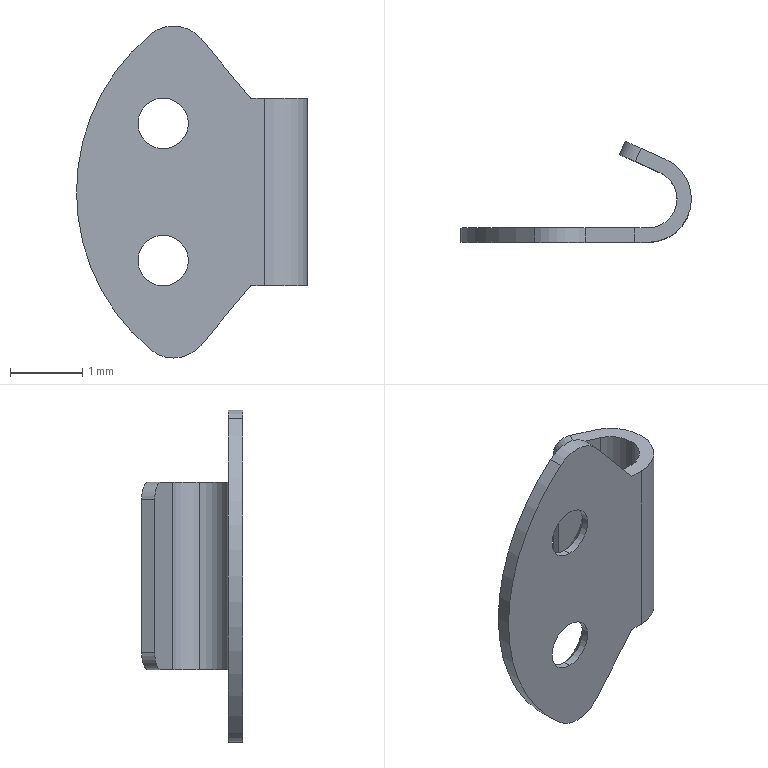Part | SolidWorks | features BaseBody 1, Scale 1 | 1 solid | 27 faces | box 3.2 x 1.4 x 4.6 mm | volume 2.668 mm3 | cylinder 14 | plane 9 | cone 4 | commonest cylinder face diameters 0.7 x4 1 x3 0.48 x2 0.8 x2 1.2 x2 5.686 x1
STEP:
#1=CARTESIAN_POINT('',(-19.88,-47.67,-12.1));
#2=VERTEX_POINT('',#1);
#3=CARTESIAN_POINT('',(-19.88,-47.67,-12.8));
#4=VERTEX_POINT('',#3);
#5=CARTESIAN_POINT('',(-19.88,-47.67,-12.45));
#6=DIRECTION('',(0.,-1.,0.));
#7=DIRECTION('',(0.,0.,1.));
#8=AXIS2_PLACEMENT_3D('',#5,#6,#7);
#9=CIRCLE('',#8,0.35);
#10=EDGE_CURVE('',#2,#4,#9,.T.);
#11=ORIENTED_EDGE('',*,*,#10,.T.);
#12=CARTESIAN_POINT('',(-19.88,-47.57,-12.9));
#13=VERTEX_POINT('',#12);
#14=CARTESIAN_POINT('',(-19.88,-47.67,-12.8));
#15=DIRECTION('',(0.,0.7071,-0.7071));
#16=VECTOR('',#15,1000.);
#17=LINE('',#14,#16);
#18=EDGE_CURVE('',#4,#13,#17,.T.);
#19=ORIENTED_EDGE('',*,*,#18,.T.);
#20=CARTESIAN_POINT('',(-19.88,-47.57,-12.));
#21=VERTEX_POINT('',#20);
#22=CARTESIAN_POINT('',(-19.88,-47.57,-12.45));
#23=DIRECTION('',(0.,1.,0.));
#24=DIRECTION('',(0.,0.,1.));
#25=AXIS2_PLACEMENT_3D('',#22,#23,#24);
#26=CIRCLE('',#25,0.45);
#27=EDGE_CURVE('',#13,#21,#26,.T.);
#28=ORIENTED_EDGE('',*,*,#27,.T.);
#29=CARTESIAN_POINT('',(-19.88,-47.67,-12.1));
#30=DIRECTION('',(0.,0.7071,0.7071));
#31=VECTOR('',#30,1000.);
#32=LINE('',#29,#31);
#33=EDGE_CURVE('',#2,#21,#32,.T.);
#34=ORIENTED_EDGE('',*,*,#33,.F.);
#35=EDGE_LOOP('',(#11,#19,#28,#34));
#36=FACE_OUTER_BOUND('',#35,.T.);
#37=CARTESIAN_POINT('',(-19.88,-47.67,-12.45));
#38=DIRECTION('',(0.,1.,0.));
#39=DIRECTION('',(0.,0.,1.));
#40=AXIS2_PLACEMENT_3D('',#37,#38,#39);
#41=CONICAL_SURFACE('',#40,0.35,0.7854);
#42=ADVANCED_FACE('',(#36),#41,.F.);
#43=ORIENTED_EDGE('',*,*,#10,.F.);
#44=CARTESIAN_POINT('',(-19.88,-47.77,-12.1));
#45=VERTEX_POINT('',#44);
#46=CARTESIAN_POINT('',(-19.88,-47.67,-12.1));
#47=DIRECTION('',(0.,-1.,0.));
#48=VECTOR('',#47,1000.);
#49=LINE('',#46,#48);
#50=EDGE_CURVE('',#2,#45,#49,.T.);
#51=ORIENTED_EDGE('',*,*,#50,.T.);
#52=CARTESIAN_POINT('',(-19.88,-47.77,-12.8));
#53=VERTEX_POINT('',#52);
#54=CARTESIAN_POINT('',(-19.88,-47.77,-12.45));
#55=DIRECTION('',(0.,-1.,0.));
#56=DIRECTION('',(0.,0.,-1.));
#57=AXIS2_PLACEMENT_3D('',#54,#55,#56);
#58=CIRCLE('',#57,0.35);
#59=EDGE_CURVE('',#45,#53,#58,.T.);
#60=ORIENTED_EDGE('',*,*,#59,.T.);
#61=CARTESIAN_POINT('',(-19.88,-47.67,-12.8));
#62=DIRECTION('',(0.,-1.,0.));
#63=VECTOR('',#62,1000.);
#64=LINE('',#61,#63);
#65=EDGE_CURVE('',#4,#53,#64,.T.);
#66=ORIENTED_EDGE('',*,*,#65,.F.);
#67=EDGE_LOOP('',(#43,#51,#60,#66));
#68=FACE_OUTER_BOUND('',#67,.T.);
#69=CARTESIAN_POINT('',(-19.88,-47.67,-12.45));
#70=DIRECTION('',(0.,-1.,0.));
#71=DIRECTION('',(0.,0.,-1.));
#72=AXIS2_PLACEMENT_3D('',#69,#70,#71);
#73=CYLINDRICAL_SURFACE('',#72,0.35);
#74=ADVANCED_FACE('',(#68),#73,.F.);
#75=CARTESIAN_POINT('',(-19.88,-47.67,-10.2));
#76=VERTEX_POINT('',#75);
#77=CARTESIAN_POINT('',(-19.88,-47.67,-10.9));
#78=VERTEX_POINT('',#77);
#79=CARTESIAN_POINT('',(-19.88,-47.67,-10.55));
#80=DIRECTION('',(0.,-1.,0.));
#81=DIRECTION('',(0.,0.,1.));
#82=AXIS2_PLACEMENT_3D('',#79,#80,#81);
#83=CIRCLE('',#82,0.35);
#84=EDGE_CURVE('',#76,#78,#83,.T.);
#85=ORIENTED_EDGE('',*,*,#84,.T.);
#86=CARTESIAN_POINT('',(-19.88,-47.57,-11.));
#87=VERTEX_POINT('',#86);
#88=CARTESIAN_POINT('',(-19.88,-47.67,-10.9));
#89=DIRECTION('',(0.,0.7071,-0.7071));
#90=VECTOR('',#89,1000.);
#91=LINE('',#88,#90);
#92=EDGE_CURVE('',#78,#87,#91,.T.);
#93=ORIENTED_EDGE('',*,*,#92,.T.);
#94=CARTESIAN_POINT('',(-19.88,-47.57,-10.1));
#95=VERTEX_POINT('',#94);
#96=CARTESIAN_POINT('',(-19.88,-47.57,-10.55));
#97=DIRECTION('',(0.,-1.,0.));
#98=DIRECTION('',(0.,0.,1.));
#99=AXIS2_PLACEMENT_3D('',#96,#97,#98);
#100=CIRCLE('',#99,0.45);
#101=EDGE_CURVE('',#95,#87,#100,.T.);
#102=ORIENTED_EDGE('',*,*,#101,.F.);
#103=CARTESIAN_POINT('',(-19.88,-47.67,-10.2));
#104=DIRECTION('',(0.,0.7071,0.7071));
#105=VECTOR('',#104,1000.);
#106=LINE('',#103,#105);
#107=EDGE_CURVE('',#76,#95,#106,.T.);
#108=ORIENTED_EDGE('',*,*,#107,.F.);
#109=EDGE_LOOP('',(#85,#93,#102,#108));
#110=FACE_OUTER_BOUND('',#109,.T.);
#111=CARTESIAN_POINT('',(-19.88,-47.67,-10.55));
#112=DIRECTION('',(0.,1.,0.));
#113=DIRECTION('',(0.,0.,1.));
#114=AXIS2_PLACEMENT_3D('',#111,#112,#113);
#115=CONICAL_SURFACE('',#114,0.35,0.7854);
#116=ADVANCED_FACE('',(#110),#115,.F.);
#117=CARTESIAN_POINT('',(-18.317,-46.805,-12.8));
#118=VERTEX_POINT('',#117);
#119=CARTESIAN_POINT('',(-18.08,-47.17,-12.8));
#120=VERTEX_POINT('',#119);
#121=CARTESIAN_POINT('',(-18.48,-47.17,-12.8));
#122=DIRECTION('',(0.,0.,-1.));
#123=DIRECTION('',(1.,0.,0.));
#124=AXIS2_PLACEMENT_3D('',#121,#122,#123);
#125=CIRCLE('',#124,0.4);
#126=EDGE_CURVE('',#118,#120,#125,.T.);
#127=ORIENTED_EDGE('',*,*,#126,.T.);
#128=CARTESIAN_POINT('',(-18.08,-47.17,-10.2));
#129=VERTEX_POINT('',#128);
#130=CARTESIAN_POINT('',(-18.08,-47.17,-12.8));
#131=DIRECTION('',(0.,0.,1.));
#132=VECTOR('',#131,1000.);
#133=LINE('',#130,#132);
#134=EDGE_CURVE('',#120,#129,#133,.T.);
#135=ORIENTED_EDGE('',*,*,#134,.T.);
#136=CARTESIAN_POINT('',(-18.317,-46.805,-10.2));
#137=VERTEX_POINT('',#136);
#138=CARTESIAN_POINT('',(-18.48,-47.17,-10.2));
#139=DIRECTION('',(0.,0.,1.));
#140=DIRECTION('',(1.,0.,0.));
#141=AXIS2_PLACEMENT_3D('',#138,#139,#140);
#142=CIRCLE('',#141,0.4);
#143=EDGE_CURVE('',#129,#137,#142,.T.);
#144=ORIENTED_EDGE('',*,*,#143,.T.);
#145=CARTESIAN_POINT('',(-18.317,-46.805,-11.5));
#146=DIRECTION('',(0.,0.,-1.));
#147=VECTOR('',#146,1000.);
#148=LINE('',#145,#147);
#149=EDGE_CURVE('',#137,#118,#148,.T.);
#150=ORIENTED_EDGE('',*,*,#149,.T.);
#151=EDGE_LOOP('',(#127,#135,#144,#150));
#152=FACE_OUTER_BOUND('',#151,.T.);
#153=CARTESIAN_POINT('',(-18.48,-47.17,-12.8));
#154=DIRECTION('',(0.,0.,1.));
#155=DIRECTION('',(1.,0.,0.));
#156=AXIS2_PLACEMENT_3D('',#153,#154,#155);
#157=CYLINDRICAL_SURFACE('',#156,0.4);
#158=ADVANCED_FACE('',(#152),#157,.F.);
#159=CARTESIAN_POINT('',(-19.737,-47.57,-13.8));
#160=VERTEX_POINT('',#159);
#161=CARTESIAN_POINT('',(-20.057,-47.57,-13.684));
#162=VERTEX_POINT('',#161);
#163=CARTESIAN_POINT('',(-19.737,-47.57,-13.3));
#164=DIRECTION('',(0.,1.,0.));
#165=DIRECTION('',(0.,0.,-1.));
#166=AXIS2_PLACEMENT_3D('',#163,#164,#165);
#167=CIRCLE('',#166,0.5);
#168=EDGE_CURVE('',#160,#162,#167,.T.);
#169=ORIENTED_EDGE('',*,*,#168,.F.);
#170=CARTESIAN_POINT('',(-19.737,-47.77,-13.8));
#171=VERTEX_POINT('',#170);
#172=CARTESIAN_POINT('',(-19.737,-47.57,-13.8));
#173=DIRECTION('',(0.,-1.,0.));
#174=VECTOR('',#173,1000.);
#175=LINE('',#172,#174);
#176=EDGE_CURVE('',#160,#171,#175,.T.);
#177=ORIENTED_EDGE('',*,*,#176,.T.);
#178=CARTESIAN_POINT('',(-20.057,-47.77,-13.684));
#179=VERTEX_POINT('',#178);
#180=CARTESIAN_POINT('',(-19.737,-47.77,-13.3));
#181=DIRECTION('',(0.,-1.,0.));
#182=DIRECTION('',(0.,0.,-1.));
#183=AXIS2_PLACEMENT_3D('',#180,#181,#182);
#184=CIRCLE('',#183,0.5);
#185=EDGE_CURVE('',#179,#171,#184,.T.);
#186=ORIENTED_EDGE('',*,*,#185,.F.);
#187=CARTESIAN_POINT('',(-20.057,-47.67,-13.684));
#188=DIRECTION('',(0.,1.,0.));
#189=VECTOR('',#188,1000.);
#190=LINE('',#187,#189);
#191=EDGE_CURVE('',#179,#162,#190,.T.);
#192=ORIENTED_EDGE('',*,*,#191,.T.);
#193=EDGE_LOOP('',(#169,#177,#186,#192));
#194=FACE_OUTER_BOUND('',#193,.T.);
#195=CARTESIAN_POINT('',(-19.737,-47.57,-13.3));
#196=DIRECTION('',(0.,-1.,0.));
#197=DIRECTION('',(0.,0.,-1.));
#198=AXIS2_PLACEMENT_3D('',#195,#196,#197);
#199=CYLINDRICAL_SURFACE('',#198,0.5);
#200=ADVANCED_FACE('',(#194),#199,.T.);
#201=ORIENTED_EDGE('',*,*,#84,.F.);
#202=CARTESIAN_POINT('',(-19.88,-47.77,-10.2));
#203=VERTEX_POINT('',#202);
#204=CARTESIAN_POINT('',(-19.88,-47.67,-10.2));
#205=DIRECTION('',(0.,-1.,0.));
#206=VECTOR('',#205,1000.);
#207=LINE('',#204,#206);
#208=EDGE_CURVE('',#76,#203,#207,.T.);
#209=ORIENTED_EDGE('',*,*,#208,.T.);
#210=CARTESIAN_POINT('',(-19.88,-47.77,-10.9));
#211=VERTEX_POINT('',#210);
#212=CARTESIAN_POINT('',(-19.88,-47.77,-10.55));
#213=DIRECTION('',(0.,1.,0.));
#214=DIRECTION('',(0.,0.,-1.));
#215=AXIS2_PLACEMENT_3D('',#212,#213,#214);
#216=CIRCLE('',#215,0.35);
#217=EDGE_CURVE('',#211,#203,#216,.T.);
#218=ORIENTED_EDGE('',*,*,#217,.F.);
#219=CARTESIAN_POINT('',(-19.88,-47.67,-10.9));
#220=DIRECTION('',(0.,-1.,0.));
#221=VECTOR('',#220,1000.);
#222=LINE('',#219,#221);
#223=EDGE_CURVE('',#78,#211,#222,.T.);
#224=ORIENTED_EDGE('',*,*,#223,.F.);
#225=EDGE_LOOP('',(#201,#209,#218,#224));
#226=FACE_OUTER_BOUND('',#225,.T.);
#227=CARTESIAN_POINT('',(-19.88,-47.67,-10.55));
#228=DIRECTION('',(0.,-1.,0.));
#229=DIRECTION('',(0.,0.,-1.));
#230=AXIS2_PLACEMENT_3D('',#227,#228,#229);
#231=CYLINDRICAL_SURFACE('',#230,0.35);
#232=ADVANCED_FACE('',(#226),#231,.F.);
#233=CARTESIAN_POINT('',(-18.48,-47.77,-12.8));
#234=VERTEX_POINT('',#233);
#235=CARTESIAN_POINT('',(-17.88,-47.17,-12.8));
#236=VERTEX_POINT('',#235);
#237=CARTESIAN_POINT('',(-18.48,-47.17,-12.8));
#238=DIRECTION('',(0.,0.,1.));
#239=DIRECTION('',(1.,0.,0.));
#240=AXIS2_PLACEMENT_3D('',#237,#238,#239);
#241=CIRCLE('',#240,0.6);
#242=EDGE_CURVE('',#234,#236,#241,.T.);
#243=ORIENTED_EDGE('',*,*,#242,.T.);
#244=CARTESIAN_POINT('',(-17.88,-47.17,-10.2));
#245=VERTEX_POINT('',#244);
#246=CARTESIAN_POINT('',(-17.88,-47.17,-12.8));
#247=DIRECTION('',(0.,0.,1.));
#248=VECTOR('',#247,1000.);
#249=LINE('',#246,#248);
#250=EDGE_CURVE('',#236,#245,#249,.T.);
#251=ORIENTED_EDGE('',*,*,#250,.T.);
#252=CARTESIAN_POINT('',(-18.48,-47.77,-10.2));
#253=VERTEX_POINT('',#252);
#254=CARTESIAN_POINT('',(-18.48,-47.17,-10.2));
#255=DIRECTION('',(0.,0.,-1.));
#256=DIRECTION('',(1.,0.,0.));
#257=AXIS2_PLACEMENT_3D('',#254,#255,#256);
#258=CIRCLE('',#257,0.6);
#259=EDGE_CURVE('',#245,#253,#258,.T.);
#260=ORIENTED_EDGE('',*,*,#259,.T.);
#261=CARTESIAN_POINT('',(-18.48,-47.77,-11.5));
#262=DIRECTION('',(0.,0.,1.));
#263=VECTOR('',#262,1000.);
#264=LINE('',#261,#263);
#265=EDGE_CURVE('',#234,#253,#264,.T.);
#266=ORIENTED_EDGE('',*,*,#265,.F.);
#267=EDGE_LOOP('',(#243,#251,#260,#266));
#268=FACE_OUTER_BOUND('',#267,.T.);
#269=CARTESIAN_POINT('',(-18.48,-47.17,-12.8));
#270=DIRECTION('',(0.,0.,1.));
#271=DIRECTION('',(1.,0.,0.));
#272=AXIS2_PLACEMENT_3D('',#269,#270,#271);
#273=CYLINDRICAL_SURFACE('',#272,0.6);
#274=ADVANCED_FACE('',(#268),#273,.T.);
#275=ORIENTED_EDGE('',*,*,#18,.F.);
#276=CARTESIAN_POINT('',(-19.88,-47.67,-12.45));
#277=DIRECTION('',(0.,-1.,0.));
#278=DIRECTION('',(0.,0.,1.));
#279=AXIS2_PLACEMENT_3D('',#276,#277,#278);
#280=CIRCLE('',#279,0.35);
#281=EDGE_CURVE('',#4,#2,#280,.T.);
#282=ORIENTED_EDGE('',*,*,#281,.T.);
#283=ORIENTED_EDGE('',*,*,#33,.T.);
#284=CARTESIAN_POINT('',(-19.88,-47.57,-12.45));
#285=DIRECTION('',(0.,1.,0.));
#286=DIRECTION('',(0.,0.,1.));
#287=AXIS2_PLACEMENT_3D('',#284,#285,#286);
#288=CIRCLE('',#287,0.45);
#289=EDGE_CURVE('',#21,#13,#288,.T.);
#290=ORIENTED_EDGE('',*,*,#289,.T.);
#291=EDGE_LOOP('',(#275,#282,#283,#290));
#292=FACE_OUTER_BOUND('',#291,.T.);
#293=CARTESIAN_POINT('',(-19.88,-47.67,-12.45));
#294=DIRECTION('',(0.,1.,0.));
#295=DIRECTION('',(0.,0.,1.));
#296=AXIS2_PLACEMENT_3D('',#293,#294,#295);
#297=CONICAL_SURFACE('',#296,0.35,0.7854);
#298=ADVANCED_FACE('',(#292),#297,.F.);
#299=ORIENTED_EDGE('',*,*,#289,.F.);
#300=ORIENTED_EDGE('',*,*,#27,.F.);
#301=EDGE_LOOP('',(#299,#300));
#302=FACE_BOUND('',#301,.T.);
#303=ORIENTED_EDGE('',*,*,#101,.T.);
#304=CARTESIAN_POINT('',(-19.88,-47.57,-10.55));
#305=DIRECTION('',(0.,-1.,0.));
#306=DIRECTION('',(0.,0.,1.));
#307=AXIS2_PLACEMENT_3D('',#304,#305,#306);
#308=CIRCLE('',#307,0.45);
#309=EDGE_CURVE('',#87,#95,#308,.T.);
#310=ORIENTED_EDGE('',*,*,#309,.T.);
#311=EDGE_LOOP('',(#303,#310));
#312=FACE_BOUND('',#311,.T.);
#313=CARTESIAN_POINT('',(-18.665,-47.57,-10.2));
#314=VERTEX_POINT('',#313);
#315=CARTESIAN_POINT('',(-18.48,-47.57,-10.2));
#316=VERTEX_POINT('',#315);
#317=CARTESIAN_POINT('',(-18.27,-47.57,-10.2));
#318=DIRECTION('',(1.,0.,0.));
#319=VECTOR('',#318,1000.);
#320=LINE('',#317,#319);
#321=EDGE_CURVE('',#314,#316,#320,.T.);
#322=ORIENTED_EDGE('',*,*,#321,.T.);
#323=CARTESIAN_POINT('',(-18.48,-47.57,-12.8));
#324=VERTEX_POINT('',#323);
#325=CARTESIAN_POINT('',(-18.48,-47.57,-11.5));
#326=DIRECTION('',(0.,0.,-1.));
#327=VECTOR('',#326,1000.);
#328=LINE('',#325,#327);
#329=EDGE_CURVE('',#316,#324,#328,.T.);
#330=ORIENTED_EDGE('',*,*,#329,.T.);
#331=CARTESIAN_POINT('',(-18.665,-47.57,-12.8));
#332=VERTEX_POINT('',#331);
#333=CARTESIAN_POINT('',(-18.27,-47.57,-12.8));
#334=DIRECTION('',(-1.,0.,0.));
#335=VECTOR('',#334,1000.);
#336=LINE('',#333,#335);
#337=EDGE_CURVE('',#324,#332,#336,.T.);
#338=ORIENTED_EDGE('',*,*,#337,.T.);
#339=CARTESIAN_POINT('',(-19.354,-47.57,-13.621));
#340=VERTEX_POINT('',#339);
#341=CARTESIAN_POINT('',(-18.665,-47.57,-12.8));
#342=DIRECTION('',(-0.6428,0.,-0.766));
#343=VECTOR('',#342,1000.);
#344=LINE('',#341,#343);
#345=EDGE_CURVE('',#332,#340,#344,.T.);
#346=ORIENTED_EDGE('',*,*,#345,.T.);
#347=CARTESIAN_POINT('',(-19.737,-47.57,-13.3));
#348=DIRECTION('',(0.,1.,0.));
#349=DIRECTION('',(0.,0.,-1.));
#350=AXIS2_PLACEMENT_3D('',#347,#348,#349);
#351=CIRCLE('',#350,0.5);
#352=EDGE_CURVE('',#340,#160,#351,.T.);
#353=ORIENTED_EDGE('',*,*,#352,.T.);
#354=ORIENTED_EDGE('',*,*,#168,.T.);
#355=CARTESIAN_POINT('',(-20.057,-47.57,-9.316));
#356=VERTEX_POINT('',#355);
#357=CARTESIAN_POINT('',(-18.237,-47.57,-11.5));
#358=DIRECTION('',(0.,1.,0.));
#359=DIRECTION('',(0.,0.,-1.));
#360=AXIS2_PLACEMENT_3D('',#357,#358,#359);
#361=CIRCLE('',#360,2.843);
#362=EDGE_CURVE('',#162,#356,#361,.T.);
#363=ORIENTED_EDGE('',*,*,#362,.T.);
#364=CARTESIAN_POINT('',(-19.354,-47.57,-9.379));
#365=VERTEX_POINT('',#364);
#366=CARTESIAN_POINT('',(-19.737,-47.57,-9.7));
#367=DIRECTION('',(0.,1.,0.));
#368=DIRECTION('',(0.,0.,-1.));
#369=AXIS2_PLACEMENT_3D('',#366,#367,#368);
#370=CIRCLE('',#369,0.5);
#371=EDGE_CURVE('',#356,#365,#370,.T.);
#372=ORIENTED_EDGE('',*,*,#371,.T.);
#373=CARTESIAN_POINT('',(-19.354,-47.57,-9.379));
#374=DIRECTION('',(0.6428,0.,-0.766));
#375=VECTOR('',#374,1000.);
#376=LINE('',#373,#375);
#377=EDGE_CURVE('',#365,#314,#376,.T.);
#378=ORIENTED_EDGE('',*,*,#377,.T.);
#379=EDGE_LOOP('',(#322,#330,#338,#346,#353,#354,#363,#372,#378));
#380=FACE_OUTER_BOUND('',#379,.T.);
#381=CARTESIAN_POINT('',(-18.48,-47.57,-13.828));
#382=DIRECTION('',(0.,1.,0.));
#383=DIRECTION('',(-1.,0.,0.));
#384=AXIS2_PLACEMENT_3D('',#381,#382,#383);
#385=PLANE('',#384);
#386=ADVANCED_FACE('',(#302,#312,#380),#385,.T.);
#387=ORIENTED_EDGE('',*,*,#50,.F.);
#388=ORIENTED_EDGE('',*,*,#281,.F.);
#389=ORIENTED_EDGE('',*,*,#65,.T.);
#390=CARTESIAN_POINT('',(-19.88,-47.77,-12.45));
#391=DIRECTION('',(0.,-1.,0.));
#392=DIRECTION('',(0.,0.,-1.));
#393=AXIS2_PLACEMENT_3D('',#390,#391,#392);
#394=CIRCLE('',#393,0.35);
#395=EDGE_CURVE('',#53,#45,#394,.T.);
#396=ORIENTED_EDGE('',*,*,#395,.T.);
#397=EDGE_LOOP('',(#387,#388,#389,#396));
#398=FACE_OUTER_BOUND('',#397,.T.);
#399=CARTESIAN_POINT('',(-19.88,-47.67,-12.45));
#400=DIRECTION('',(0.,-1.,0.));
#401=DIRECTION('',(0.,0.,-1.));
#402=AXIS2_PLACEMENT_3D('',#399,#400,#401);
#403=CYLINDRICAL_SURFACE('',#402,0.35);
#404=ADVANCED_FACE('',(#398),#403,.F.);
#405=ORIENTED_EDGE('',*,*,#92,.F.);
#406=CARTESIAN_POINT('',(-19.88,-47.67,-10.55));
#407=DIRECTION('',(0.,-1.,0.));
#408=DIRECTION('',(0.,0.,1.));
#409=AXIS2_PLACEMENT_3D('',#406,#407,#408);
#410=CIRCLE('',#409,0.35);
#411=EDGE_CURVE('',#78,#76,#410,.T.);
#412=ORIENTED_EDGE('',*,*,#411,.T.);
#413=ORIENTED_EDGE('',*,*,#107,.T.);
#414=ORIENTED_EDGE('',*,*,#309,.F.);
#415=EDGE_LOOP('',(#405,#412,#413,#414));
#416=FACE_OUTER_BOUND('',#415,.T.);
#417=CARTESIAN_POINT('',(-19.88,-47.67,-10.55));
#418=DIRECTION('',(0.,1.,0.));
#419=DIRECTION('',(0.,0.,1.));
#420=AXIS2_PLACEMENT_3D('',#417,#418,#419);
#421=CONICAL_SURFACE('',#420,0.35,0.7854);
#422=ADVANCED_FACE('',(#416),#421,.F.);
#423=ORIENTED_EDGE('',*,*,#134,.F.);
#424=CARTESIAN_POINT('',(-18.48,-47.17,-12.8));
#425=DIRECTION('',(0.,0.,-1.));
#426=DIRECTION('',(1.,0.,0.));
#427=AXIS2_PLACEMENT_3D('',#424,#425,#426);
#428=CIRCLE('',#427,0.4);
#429=EDGE_CURVE('',#120,#324,#428,.T.);
#430=ORIENTED_EDGE('',*,*,#429,.T.);
#431=ORIENTED_EDGE('',*,*,#329,.F.);
#432=CARTESIAN_POINT('',(-18.48,-47.17,-10.2));
#433=DIRECTION('',(0.,0.,1.));
#434=DIRECTION('',(1.,0.,0.));
#435=AXIS2_PLACEMENT_3D('',#432,#433,#434);
#436=CIRCLE('',#435,0.4);
#437=EDGE_CURVE('',#316,#129,#436,.T.);
#438=ORIENTED_EDGE('',*,*,#437,.T.);
#439=EDGE_LOOP('',(#423,#430,#431,#438));
#440=FACE_OUTER_BOUND('',#439,.T.);
#441=CARTESIAN_POINT('',(-18.48,-47.17,-12.8));
#442=DIRECTION('',(0.,0.,1.));
#443=DIRECTION('',(1.,0.,0.));
#444=AXIS2_PLACEMENT_3D('',#441,#442,#443);
#445=CYLINDRICAL_SURFACE('',#444,0.4);
#446=ADVANCED_FACE('',(#440),#445,.F.);
#447=CARTESIAN_POINT('',(-19.354,-47.77,-9.379));
#448=VERTEX_POINT('',#447);
#449=CARTESIAN_POINT('',(-19.354,-47.67,-9.379));
#450=DIRECTION('',(0.,1.,0.));
#451=VECTOR('',#450,1000.);
#452=LINE('',#449,#451);
#453=EDGE_CURVE('',#448,#365,#452,.T.);
#454=ORIENTED_EDGE('',*,*,#453,.F.);
#455=CARTESIAN_POINT('',(-18.665,-47.77,-10.2));
#456=VERTEX_POINT('',#455);
#457=CARTESIAN_POINT('',(-19.009,-47.77,-9.789));
#458=DIRECTION('',(-0.6428,0.,0.766));
#459=VECTOR('',#458,1000.);
#460=LINE('',#457,#459);
#461=EDGE_CURVE('',#456,#448,#460,.T.);
#462=ORIENTED_EDGE('',*,*,#461,.F.);
#463=CARTESIAN_POINT('',(-18.665,-47.67,-10.2));
#464=DIRECTION('',(0.,-1.,0.));
#465=VECTOR('',#464,1000.);
#466=LINE('',#463,#465);
#467=EDGE_CURVE('',#314,#456,#466,.T.);
#468=ORIENTED_EDGE('',*,*,#467,.F.);
#469=ORIENTED_EDGE('',*,*,#377,.F.);
#470=EDGE_LOOP('',(#454,#462,#468,#469));
#471=FACE_OUTER_BOUND('',#470,.T.);
#472=CARTESIAN_POINT('',(-18.665,-47.77,-10.2));
#473=DIRECTION('',(-0.766,0.,-0.6428));
#474=DIRECTION('',(-0.6428,0.,0.766));
#475=AXIS2_PLACEMENT_3D('',#472,#473,#474);
#476=PLANE('',#475);
#477=ADVANCED_FACE('',(#471),#476,.F.);
#478=CARTESIAN_POINT('',(-20.057,-47.77,-9.316));
#479=VERTEX_POINT('',#478);
#480=CARTESIAN_POINT('',(-20.057,-47.67,-9.316));
#481=DIRECTION('',(0.,1.,0.));
#482=VECTOR('',#481,1000.);
#483=LINE('',#480,#482);
#484=EDGE_CURVE('',#479,#356,#483,.T.);
#485=ORIENTED_EDGE('',*,*,#484,.F.);
#486=CARTESIAN_POINT('',(-19.737,-47.77,-9.7));
#487=DIRECTION('',(0.,-1.,0.));
#488=DIRECTION('',(0.,0.,-1.));
#489=AXIS2_PLACEMENT_3D('',#486,#487,#488);
#490=CIRCLE('',#489,0.5);
#491=EDGE_CURVE('',#448,#479,#490,.T.);
#492=ORIENTED_EDGE('',*,*,#491,.F.);
#493=ORIENTED_EDGE('',*,*,#453,.T.);
#494=ORIENTED_EDGE('',*,*,#371,.F.);
#495=EDGE_LOOP('',(#485,#492,#493,#494));
#496=FACE_OUTER_BOUND('',#495,.T.);
#497=CARTESIAN_POINT('',(-19.737,-47.57,-9.7));
#498=DIRECTION('',(0.,-1.,0.));
#499=DIRECTION('',(0.,0.,-1.));
#500=AXIS2_PLACEMENT_3D('',#497,#498,#499);
#501=CYLINDRICAL_SURFACE('',#500,0.5);
#502=ADVANCED_FACE('',(#496),#501,.T.);
#503=ORIENTED_EDGE('',*,*,#191,.F.);
#504=CARTESIAN_POINT('',(-18.237,-47.77,-11.5));
#505=DIRECTION('',(0.,-1.,0.));
#506=DIRECTION('',(0.,0.,-1.));
#507=AXIS2_PLACEMENT_3D('',#504,#505,#506);
#508=CIRCLE('',#507,2.843);
#509=EDGE_CURVE('',#479,#179,#508,.T.);
#510=ORIENTED_EDGE('',*,*,#509,.F.);
#511=ORIENTED_EDGE('',*,*,#484,.T.);
#512=ORIENTED_EDGE('',*,*,#362,.F.);
#513=EDGE_LOOP('',(#503,#510,#511,#512));
#514=FACE_OUTER_BOUND('',#513,.T.);
#515=CARTESIAN_POINT('',(-18.237,-47.57,-11.5));
#516=DIRECTION('',(0.,-1.,0.));
#517=DIRECTION('',(0.,0.,-1.));
#518=AXIS2_PLACEMENT_3D('',#515,#516,#517);
#519=CYLINDRICAL_SURFACE('',#518,2.843);
#520=ADVANCED_FACE('',(#514),#519,.T.);
#521=ORIENTED_EDGE('',*,*,#176,.F.);
#522=ORIENTED_EDGE('',*,*,#352,.F.);
#523=CARTESIAN_POINT('',(-19.354,-47.77,-13.621));
#524=VERTEX_POINT('',#523);
#525=CARTESIAN_POINT('',(-19.354,-47.67,-13.621));
#526=DIRECTION('',(0.,1.,0.));
#527=VECTOR('',#526,1000.);
#528=LINE('',#525,#527);
#529=EDGE_CURVE('',#524,#340,#528,.T.);
#530=ORIENTED_EDGE('',*,*,#529,.F.);
#531=CARTESIAN_POINT('',(-19.737,-47.77,-13.3));
#532=DIRECTION('',(0.,-1.,0.));
#533=DIRECTION('',(0.,0.,-1.));
#534=AXIS2_PLACEMENT_3D('',#531,#532,#533);
#535=CIRCLE('',#534,0.5);
#536=EDGE_CURVE('',#171,#524,#535,.T.);
#537=ORIENTED_EDGE('',*,*,#536,.F.);
#538=EDGE_LOOP('',(#521,#522,#530,#537));
#539=FACE_OUTER_BOUND('',#538,.T.);
#540=CARTESIAN_POINT('',(-19.737,-47.57,-13.3));
#541=DIRECTION('',(0.,-1.,0.));
#542=DIRECTION('',(0.,0.,-1.));
#543=AXIS2_PLACEMENT_3D('',#540,#541,#542);
#544=CYLINDRICAL_SURFACE('',#543,0.5);
#545=ADVANCED_FACE('',(#539),#544,.T.);
#546=CARTESIAN_POINT('',(-18.665,-47.77,-12.8));
#547=VERTEX_POINT('',#546);
#548=CARTESIAN_POINT('',(-18.665,-47.67,-12.8));
#549=DIRECTION('',(0.,1.,0.));
#550=VECTOR('',#549,1000.);
#551=LINE('',#548,#550);
#552=EDGE_CURVE('',#547,#332,#551,.T.);
#553=ORIENTED_EDGE('',*,*,#552,.F.);
#554=CARTESIAN_POINT('',(-19.009,-47.77,-13.211));
#555=DIRECTION('',(0.6428,0.,0.766));
#556=VECTOR('',#555,1000.);
#557=LINE('',#554,#556);
#558=EDGE_CURVE('',#524,#547,#557,.T.);
#559=ORIENTED_EDGE('',*,*,#558,.F.);
#560=ORIENTED_EDGE('',*,*,#529,.T.);
#561=ORIENTED_EDGE('',*,*,#345,.F.);
#562=EDGE_LOOP('',(#553,#559,#560,#561));
#563=FACE_OUTER_BOUND('',#562,.T.);
#564=CARTESIAN_POINT('',(-19.354,-47.77,-13.621));
#565=DIRECTION('',(-0.766,0.,0.6428));
#566=DIRECTION('',(0.6428,0.,0.766));
#567=AXIS2_PLACEMENT_3D('',#564,#565,#566);
#568=PLANE('',#567);
#569=ADVANCED_FACE('',(#563),#568,.F.);
#570=ORIENTED_EDGE('',*,*,#217,.T.);
#571=CARTESIAN_POINT('',(-19.88,-47.77,-10.55));
#572=DIRECTION('',(0.,1.,0.));
#573=DIRECTION('',(0.,0.,-1.));
#574=AXIS2_PLACEMENT_3D('',#571,#572,#573);
#575=CIRCLE('',#574,0.35);
#576=EDGE_CURVE('',#203,#211,#575,.T.);
#577=ORIENTED_EDGE('',*,*,#576,.T.);
#578=EDGE_LOOP('',(#570,#577));
#579=FACE_BOUND('',#578,.T.);
#580=ORIENTED_EDGE('',*,*,#395,.F.);
#581=ORIENTED_EDGE('',*,*,#59,.F.);
#582=EDGE_LOOP('',(#580,#581));
#583=FACE_BOUND('',#582,.T.);
#584=ORIENTED_EDGE('',*,*,#185,.T.);
#585=ORIENTED_EDGE('',*,*,#536,.T.);
#586=ORIENTED_EDGE('',*,*,#558,.T.);
#587=CARTESIAN_POINT('',(-19.788,-47.77,-12.8));
#588=DIRECTION('',(1.,0.,0.));
#589=VECTOR('',#588,1000.);
#590=LINE('',#587,#589);
#591=EDGE_CURVE('',#547,#234,#590,.T.);
#592=ORIENTED_EDGE('',*,*,#591,.T.);
#593=ORIENTED_EDGE('',*,*,#265,.T.);
#594=CARTESIAN_POINT('',(-19.788,-47.77,-10.2));
#595=DIRECTION('',(-1.,0.,0.));
#596=VECTOR('',#595,1000.);
#597=LINE('',#594,#596);
#598=EDGE_CURVE('',#253,#456,#597,.T.);
#599=ORIENTED_EDGE('',*,*,#598,.T.);
#600=ORIENTED_EDGE('',*,*,#461,.T.);
#601=ORIENTED_EDGE('',*,*,#491,.T.);
#602=ORIENTED_EDGE('',*,*,#509,.T.);
#603=EDGE_LOOP('',(#584,#585,#586,#592,#593,#599,#600,#601,#602));
#604=FACE_OUTER_BOUND('',#603,.T.);
#605=CARTESIAN_POINT('',(-21.096,-47.77,-13.828));
#606=DIRECTION('',(0.,-1.,0.));
#607=DIRECTION('',(1.,0.,0.));
#608=AXIS2_PLACEMENT_3D('',#605,#606,#607);
#609=PLANE('',#608);
#610=ADVANCED_FACE('',(#579,#583,#604),#609,.T.);
#611=ORIENTED_EDGE('',*,*,#208,.F.);
#612=ORIENTED_EDGE('',*,*,#411,.F.);
#613=ORIENTED_EDGE('',*,*,#223,.T.);
#614=ORIENTED_EDGE('',*,*,#576,.F.);
#615=EDGE_LOOP('',(#611,#612,#613,#614));
#616=FACE_OUTER_BOUND('',#615,.T.);
#617=CARTESIAN_POINT('',(-19.88,-47.67,-10.55));
#618=DIRECTION('',(0.,-1.,0.));
#619=DIRECTION('',(0.,0.,-1.));
#620=AXIS2_PLACEMENT_3D('',#617,#618,#619);
#621=CYLINDRICAL_SURFACE('',#620,0.35);
#622=ADVANCED_FACE('',(#616),#621,.F.);
#623=CARTESIAN_POINT('',(-18.579,-46.468,-10.2));
#624=VERTEX_POINT('',#623);
#625=CARTESIAN_POINT('',(-18.661,-46.65,-10.2));
#626=VERTEX_POINT('',#625);
#627=CARTESIAN_POINT('',(-18.62,-46.559,-10.2));
#628=DIRECTION('',(-0.4086,-0.9127,-0.000000001));
#629=VECTOR('',#628,1000.);
#630=LINE('',#627,#629);
#631=EDGE_CURVE('',#624,#626,#630,.T.);
#632=ORIENTED_EDGE('',*,*,#631,.T.);
#633=CARTESIAN_POINT('',(-18.88,-46.552,-10.2));
#634=DIRECTION('',(-0.9127,0.4086,0.));
#635=VECTOR('',#634,1000.);
#636=LINE('',#633,#635);
#637=EDGE_CURVE('',#137,#626,#636,.T.);
#638=ORIENTED_EDGE('',*,*,#637,.F.);
#639=ORIENTED_EDGE('',*,*,#143,.F.);
#640=ORIENTED_EDGE('',*,*,#437,.F.);
#641=ORIENTED_EDGE('',*,*,#321,.F.);
#642=ORIENTED_EDGE('',*,*,#467,.T.);
#643=ORIENTED_EDGE('',*,*,#598,.F.);
#644=ORIENTED_EDGE('',*,*,#259,.F.);
#645=CARTESIAN_POINT('',(-18.235,-46.622,-10.2));
#646=VERTEX_POINT('',#645);
#647=CARTESIAN_POINT('',(-18.48,-47.17,-10.2));
#648=DIRECTION('',(0.,0.,-1.));
#649=DIRECTION('',(1.,0.,0.));
#650=AXIS2_PLACEMENT_3D('',#647,#648,#649);
#651=CIRCLE('',#650,0.6);
#652=EDGE_CURVE('',#646,#245,#651,.T.);
#653=ORIENTED_EDGE('',*,*,#652,.F.);
#654=CARTESIAN_POINT('',(-18.235,-46.622,-10.2));
#655=DIRECTION('',(0.9127,-0.4086,0.));
#656=VECTOR('',#655,1000.);
#657=LINE('',#654,#656);
#658=EDGE_CURVE('',#624,#646,#657,.T.);
#659=ORIENTED_EDGE('',*,*,#658,.F.);
#660=EDGE_LOOP('',(#632,#638,#639,#640,#641,#642,#643,#644,#653,#659));
#661=FACE_OUTER_BOUND('',#660,.T.);
#662=CARTESIAN_POINT('',(-17.875,-47.77,-10.2));
#663=DIRECTION('',(0.,0.,-1.));
#664=DIRECTION('',(-1.,0.,0.));
#665=AXIS2_PLACEMENT_3D('',#662,#663,#664);
#666=PLANE('',#665);
#667=ADVANCED_FACE('',(#661),#666,.F.);
#668=CARTESIAN_POINT('',(-18.661,-46.65,-12.8));
#669=VERTEX_POINT('',#668);
#670=CARTESIAN_POINT('',(-18.579,-46.468,-12.8));
#671=VERTEX_POINT('',#670);
#672=CARTESIAN_POINT('',(-18.62,-46.559,-12.8));
#673=DIRECTION('',(0.4086,0.9127,-0.000000001));
#674=VECTOR('',#673,1000.);
#675=LINE('',#672,#674);
#676=EDGE_CURVE('',#669,#671,#675,.T.);
#677=ORIENTED_EDGE('',*,*,#676,.T.);
#678=CARTESIAN_POINT('',(-18.235,-46.622,-12.8));
#679=VERTEX_POINT('',#678);
#680=CARTESIAN_POINT('',(-18.235,-46.622,-12.8));
#681=DIRECTION('',(-0.9127,0.4086,0.));
#682=VECTOR('',#681,1000.);
#683=LINE('',#680,#682);
#684=EDGE_CURVE('',#679,#671,#683,.T.);
#685=ORIENTED_EDGE('',*,*,#684,.F.);
#686=CARTESIAN_POINT('',(-18.48,-47.17,-12.8));
#687=DIRECTION('',(0.,0.,1.));
#688=DIRECTION('',(1.,0.,0.));
#689=AXIS2_PLACEMENT_3D('',#686,#687,#688);
#690=CIRCLE('',#689,0.6);
#691=EDGE_CURVE('',#236,#679,#690,.T.);
#692=ORIENTED_EDGE('',*,*,#691,.F.);
#693=ORIENTED_EDGE('',*,*,#242,.F.);
#694=ORIENTED_EDGE('',*,*,#591,.F.);
#695=ORIENTED_EDGE('',*,*,#552,.T.);
#696=ORIENTED_EDGE('',*,*,#337,.F.);
#697=ORIENTED_EDGE('',*,*,#429,.F.);
#698=ORIENTED_EDGE('',*,*,#126,.F.);
#699=CARTESIAN_POINT('',(-18.88,-46.552,-12.8));
#700=DIRECTION('',(0.9127,-0.4086,0.));
#701=VECTOR('',#700,1000.);
#702=LINE('',#699,#701);
#703=EDGE_CURVE('',#669,#118,#702,.T.);
#704=ORIENTED_EDGE('',*,*,#703,.F.);
#705=EDGE_LOOP('',(#677,#685,#692,#693,#694,#695,#696,#697,#698,#704));
#706=FACE_OUTER_BOUND('',#705,.T.);
#707=CARTESIAN_POINT('',(-18.665,-47.77,-12.8));
#708=DIRECTION('',(0.,0.,1.));
#709=DIRECTION('',(1.,0.,0.));
#710=AXIS2_PLACEMENT_3D('',#707,#708,#709);
#711=PLANE('',#710);
#712=ADVANCED_FACE('',(#706),#711,.F.);
#713=ORIENTED_EDGE('',*,*,#250,.F.);
#714=ORIENTED_EDGE('',*,*,#691,.T.);
#715=CARTESIAN_POINT('',(-18.235,-46.622,-11.5));
#716=DIRECTION('',(0.,0.,-1.));
#717=VECTOR('',#716,1000.);
#718=LINE('',#715,#717);
#719=EDGE_CURVE('',#646,#679,#718,.T.);
#720=ORIENTED_EDGE('',*,*,#719,.F.);
#721=ORIENTED_EDGE('',*,*,#652,.T.);
#722=EDGE_LOOP('',(#713,#714,#720,#721));
#723=FACE_OUTER_BOUND('',#722,.T.);
#724=CARTESIAN_POINT('',(-18.48,-47.17,-12.8));
#725=DIRECTION('',(0.,0.,1.));
#726=DIRECTION('',(1.,0.,0.));
#727=AXIS2_PLACEMENT_3D('',#724,#725,#726);
#728=CYLINDRICAL_SURFACE('',#727,0.6);
#729=ADVANCED_FACE('',(#723),#728,.T.);
#730=ORIENTED_EDGE('',*,*,#658,.T.);
#731=ORIENTED_EDGE('',*,*,#719,.T.);
#732=ORIENTED_EDGE('',*,*,#684,.T.);
#733=CARTESIAN_POINT('',(-18.798,-46.37,-12.56));
#734=VERTEX_POINT('',#733);
#735=CARTESIAN_POINT('',(-18.579,-46.468,-12.56));
#736=DIRECTION('',(0.4086,0.9127,0.));
#737=DIRECTION('',(0.9127,-0.4086,0.));
#738=AXIS2_PLACEMENT_3D('',#735,#736,#737);
#739=CIRCLE('',#738,0.24);
#740=EDGE_CURVE('',#671,#734,#739,.T.);
#741=ORIENTED_EDGE('',*,*,#740,.T.);
#742=CARTESIAN_POINT('',(-18.798,-46.37,-10.44));
#743=VERTEX_POINT('',#742);
#744=CARTESIAN_POINT('',(-18.798,-46.37,-11.5));
#745=DIRECTION('',(0.,0.,1.));
#746=VECTOR('',#745,1000.);
#747=LINE('',#744,#746);
#748=EDGE_CURVE('',#734,#743,#747,.T.);
#749=ORIENTED_EDGE('',*,*,#748,.T.);
#750=CARTESIAN_POINT('',(-18.579,-46.468,-10.44));
#751=DIRECTION('',(0.4086,0.9127,0.));
#752=DIRECTION('',(-0.9127,0.4086,0.));
#753=AXIS2_PLACEMENT_3D('',#750,#751,#752);
#754=CIRCLE('',#753,0.24);
#755=EDGE_CURVE('',#743,#624,#754,.T.);
#756=ORIENTED_EDGE('',*,*,#755,.T.);
#757=EDGE_LOOP('',(#730,#731,#732,#741,#749,#756));
#758=FACE_OUTER_BOUND('',#757,.T.);
#759=CARTESIAN_POINT('',(-18.235,-46.622,-12.8));
#760=DIRECTION('',(0.4086,0.9127,0.));
#761=DIRECTION('',(-0.9127,0.4086,0.));
#762=AXIS2_PLACEMENT_3D('',#759,#760,#761);
#763=PLANE('',#762);
#764=ADVANCED_FACE('',(#758),#763,.T.);
#765=ORIENTED_EDGE('',*,*,#637,.T.);
#766=CARTESIAN_POINT('',(-18.88,-46.552,-10.44));
#767=VERTEX_POINT('',#766);
#768=CARTESIAN_POINT('',(-18.661,-46.65,-10.44));
#769=DIRECTION('',(-0.4086,-0.9127,0.));
#770=DIRECTION('',(-0.9127,0.4086,0.));
#771=AXIS2_PLACEMENT_3D('',#768,#769,#770);
#772=CIRCLE('',#771,0.24);
#773=EDGE_CURVE('',#626,#767,#772,.T.);
#774=ORIENTED_EDGE('',*,*,#773,.T.);
#775=CARTESIAN_POINT('',(-18.88,-46.552,-12.56));
#776=VERTEX_POINT('',#775);
#777=CARTESIAN_POINT('',(-18.88,-46.552,-11.5));
#778=DIRECTION('',(0.,0.,-1.));
#779=VECTOR('',#778,1000.);
#780=LINE('',#777,#779);
#781=EDGE_CURVE('',#767,#776,#780,.T.);
#782=ORIENTED_EDGE('',*,*,#781,.T.);
#783=CARTESIAN_POINT('',(-18.661,-46.65,-12.56));
#784=DIRECTION('',(-0.4086,-0.9127,0.));
#785=DIRECTION('',(0.9127,-0.4086,0.));
#786=AXIS2_PLACEMENT_3D('',#783,#784,#785);
#787=CIRCLE('',#786,0.24);
#788=EDGE_CURVE('',#776,#669,#787,.T.);
#789=ORIENTED_EDGE('',*,*,#788,.T.);
#790=ORIENTED_EDGE('',*,*,#703,.T.);
#791=ORIENTED_EDGE('',*,*,#149,.F.);
#792=EDGE_LOOP('',(#765,#774,#782,#789,#790,#791));
#793=FACE_OUTER_BOUND('',#792,.T.);
#794=CARTESIAN_POINT('',(-18.88,-46.552,-12.8));
#795=DIRECTION('',(-0.4086,-0.9127,0.));
#796=DIRECTION('',(0.9127,-0.4086,0.));
#797=AXIS2_PLACEMENT_3D('',#794,#795,#796);
#798=PLANE('',#797);
#799=ADVANCED_FACE('',(#793),#798,.T.);
#800=CARTESIAN_POINT('',(-18.839,-46.461,-10.44));
#801=DIRECTION('',(0.4086,0.9127,0.));
#802=VECTOR('',#801,1000.);
#803=LINE('',#800,#802);
#804=EDGE_CURVE('',#767,#743,#803,.T.);
#805=ORIENTED_EDGE('',*,*,#804,.F.);
#806=ORIENTED_EDGE('',*,*,#773,.F.);
#807=ORIENTED_EDGE('',*,*,#631,.F.);
#808=ORIENTED_EDGE('',*,*,#755,.F.);
#809=EDGE_LOOP('',(#805,#806,#807,#808));
#810=FACE_OUTER_BOUND('',#809,.T.);
#811=CARTESIAN_POINT('',(-18.661,-46.65,-10.44));
#812=DIRECTION('',(0.4086,0.9127,0.));
#813=DIRECTION('',(-0.9127,0.4086,0.));
#814=AXIS2_PLACEMENT_3D('',#811,#812,#813);
#815=CYLINDRICAL_SURFACE('',#814,0.24);
#816=ADVANCED_FACE('',(#810),#815,.T.);
#817=ORIENTED_EDGE('',*,*,#781,.F.);
#818=ORIENTED_EDGE('',*,*,#804,.T.);
#819=ORIENTED_EDGE('',*,*,#748,.F.);
#820=CARTESIAN_POINT('',(-18.839,-46.461,-12.56));
#821=DIRECTION('',(-0.4086,-0.9127,0.));
#822=VECTOR('',#821,1000.);
#823=LINE('',#820,#822);
#824=EDGE_CURVE('',#734,#776,#823,.T.);
#825=ORIENTED_EDGE('',*,*,#824,.T.);
#826=EDGE_LOOP('',(#817,#818,#819,#825));
#827=FACE_OUTER_BOUND('',#826,.T.);
#828=CARTESIAN_POINT('',(-18.798,-46.37,-12.56));
#829=DIRECTION('',(-0.9127,0.4086,0.));
#830=DIRECTION('',(-0.4086,-0.9127,0.));
#831=AXIS2_PLACEMENT_3D('',#828,#829,#830);
#832=PLANE('',#831);
#833=ADVANCED_FACE('',(#827),#832,.T.);
#834=ORIENTED_EDGE('',*,*,#824,.F.);
#835=ORIENTED_EDGE('',*,*,#740,.F.);
#836=ORIENTED_EDGE('',*,*,#676,.F.);
#837=ORIENTED_EDGE('',*,*,#788,.F.);
#838=EDGE_LOOP('',(#834,#835,#836,#837));
#839=FACE_OUTER_BOUND('',#838,.T.);
#840=CARTESIAN_POINT('',(-18.579,-46.468,-12.56));
#841=DIRECTION('',(-0.4086,-0.9127,0.));
#842=DIRECTION('',(0.9127,-0.4086,0.));
#843=AXIS2_PLACEMENT_3D('',#840,#841,#842);
#844=CYLINDRICAL_SURFACE('',#843,0.24);
#845=ADVANCED_FACE('',(#839),#844,.T.);
#846=CLOSED_SHELL('',(#42,#74,#116,#158,#200,#232,#274,#298,#386,#404,#422,#446,#477,#502,#520,#545,#569,#610,#622,#667,#712,#729,#764,#799,#816,#833,#845));
#847=MANIFOLD_SOLID_BREP('',#846);
#848=CARTESIAN_POINT('',(0.,0.,0.));
#849=DIRECTION('',(0.,0.,1.));
#850=DIRECTION('',(1.,0.,0.));
#851=AXIS2_PLACEMENT_3D('',#848,#849,#850);
#852=(LENGTH_UNIT()NAMED_UNIT(*)SI_UNIT(.MILLI.,.METRE.));
#853=UNCERTAINTY_MEASURE_WITH_UNIT(LENGTH_MEASURE(0.00001),#852,'','');
#854=(NAMED_UNIT(*)PLANE_ANGLE_UNIT()SI_UNIT($,.RADIAN.));
#855=(NAMED_UNIT(*)SI_UNIT($,.STERADIAN.)SOLID_ANGLE_UNIT());
#856=(GEOMETRIC_REPRESENTATION_CONTEXT(3)GLOBAL_UNCERTAINTY_ASSIGNED_CONTEXT((#853))GLOBAL_UNIT_ASSIGNED_CONTEXT((#852,#854,#855))REPRESENTATION_CONTEXT('',''));
#857=ADVANCED_BREP_SHAPE_REPRESENTATION('',(#847,#851),#856);